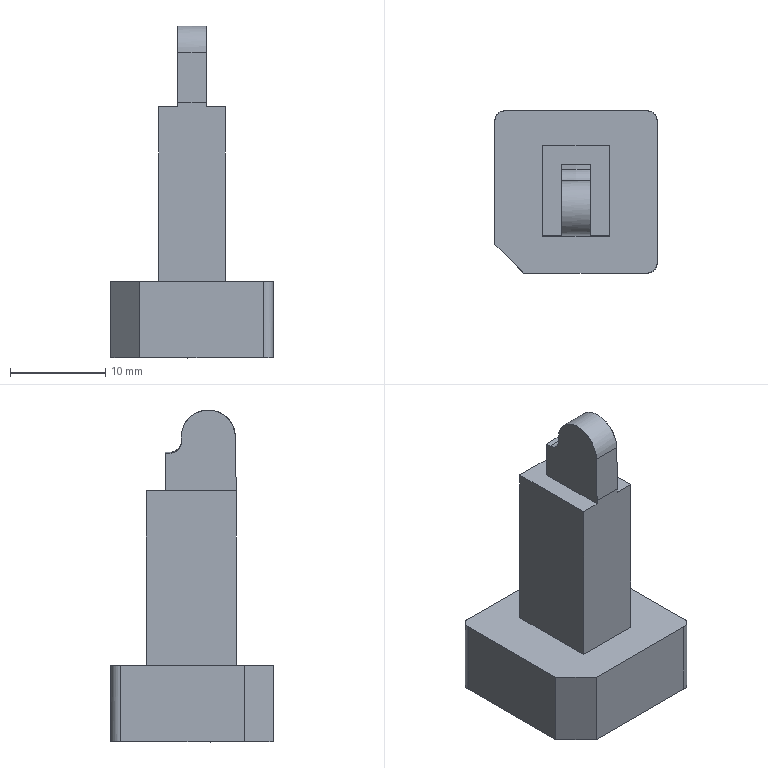NC program | PowerMill | posted with a generic post | part box 17 x 17 x 34.811 mm
Lines 20352 to 21135 of 55221:
N20449 M6
N20450 S18000 M03
N20451 G00 G90 X0.0 Y0.0
N20452 G43 Z10.798 H14
N20453
N20454 G05 P10000 R8
N20455 X2.8132 Y-4.4417
N20456 Z0.9995
N20457 G01 Z-0.2005 F1200.0
N20458 X2.7986 Y-4.3934 F2000.0
N20459 X2.7803 Y-4.3463
N20460 X2.7582 Y-4.3008
N20461 X2.7327 Y-4.2572
N20462 X2.7037 Y-4.2157
N20463 X2.6716 Y-4.1767
N20464 X2.6366 Y-4.1403
N20465 X2.5987 Y-4.1068
N20466 X2.5584 Y-4.0764
N20467 X2.5158 Y-4.0493
N20468 X2.4711 Y-4.0256
N20469 X2.4248 Y-4.0055
N20470 X2.377 Y-3.9892
N20471 X2.3281 Y-3.9766
N20472 X2.2782 Y-3.968
N20473 X2.2279 Y-3.9633
N20474 X2.1774 Y-3.9626
N20475 X2.127 Y-3.9658
N20476 X2.077 Y-3.9731
N20477 X2.0331 Y-3.9828
N20478 X1.9465 Y-4.0053
N20479 X1.8628 Y-4.0231
N20480 X1.783 Y-4.0364
N20481 X1.7026 Y-4.0459
N20482 X1.6159 Y-4.0523
N20483 X1.519 Y-4.0557
N20484 X1.4057 Y-4.0562
N20485 X0.4884 Y-4.0561
N20486 X-0.7174 Y-4.056
N20487 X-1.4208 Y-4.0571
N20488 X-1.5008 Y-4.0569
N20489 X-1.5823 Y-4.0547
N20490 X-1.6674 Y-4.0493
N20491 X-1.7533 Y-4.0404
N20492 X-1.8337 Y-4.0283
N20493 X-1.9109 Y-4.0133
N20494 X-1.9876 Y-3.9951
N20495 X-2.0635 Y-3.9738
N20496 X-2.1466 Y-3.9467
N20497 X-2.2284 Y-3.9158
N20498 X-2.3087 Y-3.8813
N20499 X-2.3874 Y-3.843
N20500 X-2.4643 Y-3.8012
N20501 X-2.5393 Y-3.756
N20502 X-2.6122 Y-3.7073
N20503 X-2.6827 Y-3.6553
N20504 X-2.7508 Y-3.6002
N20505 X-2.8164 Y-3.5421
N20506 X-2.8792 Y-3.481
N20507 X-2.9392 Y-3.4171
N20508 X-2.9963 Y-3.3505
N20509 X-3.0503 Y-3.2815
N20510 X-3.1009 Y-3.2102
N20511 X-3.1484 Y-3.1366
N20512 X-3.1924 Y-3.0609
N20513 X-3.2329 Y-2.9833
N20514 X-3.2699 Y-2.9038
N20515 X-3.3033 Y-2.8227
N20516 X-3.3329 Y-2.7401
N20517 X-3.3587 Y-2.6562
N20518 X-3.3807 Y-2.5713
N20519 X-3.3988 Y-2.4855
N20520 X-3.413 Y-2.3988
N20521 X-3.4232 Y-2.3121
N20522 X-3.4294 Y-2.2257
N20523 X-3.4316 Y-2.1396
N20524 X-3.4317 Y-2.0535
N20525 X-3.4323 Y-1.3276
N20526 X-3.4307 Y-1.2334
N20527 X-3.4253 Y-1.1417
N20528 X-3.4161 Y-1.0522
N20529 X-3.4033 Y-0.9649
N20530 X-3.3868 Y-0.8795
N20531 X-3.3667 Y-0.7958
N20532 X-3.3429 Y-0.7138
N20533 X-3.3156 Y-0.6333
N20534 X-3.2838 Y-0.5518
N20535 X-3.2483 Y-0.4718
N20536 X-3.2092 Y-0.3935
N20537 X-3.1666 Y-0.3171
N20538 X-3.1205 Y-0.2426
N20539 X-3.0711 Y-0.1702
N20540 X-3.0184 Y-0.1002
N20541 X-2.9625 Y-0.0325
N20542 X-2.9036 Y0.0325
N20543 X-2.8418 Y0.0948
N20544 X-2.7773 Y0.1542
N20545 X-2.7101 Y0.2106
N20546 X-2.6405 Y0.2638
N20547 X-2.5686 Y0.3137
N20548 X-2.4946 Y0.3603
N20549 X-2.4185 Y0.4035
N20550 X-2.3405 Y0.4431
N20551 X-2.2608 Y0.4792
N20552 X-2.1795 Y0.5116
N20553 X-2.1011 Y0.5389
N20554 X-2.0215 Y0.5628
N20555 X-1.9398 Y0.5833
N20556 X-1.8556 Y0.6004
N20557 X-1.7687 Y0.614
N20558 X-1.6787 Y0.6242
N20559 X-1.5853 Y0.6308
N20560 X-1.4884 Y0.634
N20561 X-1.3882 Y0.6342
N20562 X0.0 Y0.6333
N20563 X0.8605 Y0.6327
N20564 X1.4431 Y0.6342
N20565 X1.5395 Y0.6331
N20566 X1.6329 Y0.6284
N20567 X1.7234 Y0.6202
N20568 X1.811 Y0.6084
N20569 X1.8959 Y0.5931
N20570 X1.9784 Y0.5743
N20571 X2.0587 Y0.5522
N20572 X2.1376 Y0.5268
N20573 X2.2195 Y0.4963
N20574 X2.2999 Y0.4621
N20575 X2.3788 Y0.4243
N20576 X2.4559 Y0.3828
N20577 X2.5312 Y0.3378
N20578 X2.6044 Y0.2894
N20579 X2.6752 Y0.2378
N20580 X2.7437 Y0.1829
N20581 X2.8097 Y0.125
N20582 X2.873 Y0.0641
N20583 X2.9334 Y0.0004
N20584 X2.9909 Y-0.0659
N20585 X3.0452 Y-0.1347
N20586 X3.0962 Y-0.2058
N20587 X3.1439 Y-0.2791
N20588 X3.1882 Y-0.3544
N20589 X3.229 Y-0.4317
N20590 X3.2662 Y-0.5107
N20591 X3.2988 Y-0.589
N20592 X3.3279 Y-0.6691
N20593 X3.3544 Y-0.7532
N20594 X3.3782 Y-0.842
N20595 X3.3898 Y-0.8923
N20596 X3.3997 Y-0.9429
N20597 X3.4083 Y-0.9938
N20598 X3.4176 Y-1.0584
N20599 X3.4236 Y-1.1096
N20600 X3.428 Y-1.161
N20601 X3.4301 Y-1.2124
N20602 X3.4314 Y-1.4233
N20603 X3.4316 Y-1.6341
N20604 X3.4319 Y-2.069
N20605 X3.4316 Y-2.1567
N20606 X3.4284 Y-2.2443
N20607 X3.4212 Y-2.3316
N20608 X3.4101 Y-2.4185
N20609 X3.395 Y-2.5049
N20610 X3.3761 Y-2.5904
N20611 X3.3532 Y-2.6751
N20612 X3.3265 Y-2.7586
N20613 X3.296 Y-2.8409
N20614 X3.2618 Y-2.9218
N20615 X3.224 Y-3.001
N20616 X3.1826 Y-3.0783
N20617 X3.1377 Y-3.1537
N20618 X3.0895 Y-3.2269
N20619 X3.038 Y-3.2978
N20620 X2.9834 Y-3.3663
N20621 X2.9256 Y-3.4322
N20622 X2.865 Y-3.4955
N20623 X2.8021 Y-3.5554
N20624 X2.7364 Y-3.6125
N20625 X2.6678 Y-3.6668
N20626 X2.5966 Y-3.7181
N20627 X2.523 Y-3.7662
N20628 X2.4473 Y-3.8109
N20629 X2.3697 Y-3.8521
N20630 X2.2906 Y-3.8896
N20631 X2.2101 Y-3.9233
N20632 X2.1286 Y-3.9531
N20633 X2.0463 Y-3.9791
N20634 X2.0331 Y-3.9828
N20635 X1.966 Y-3.9991 Z-0.2006
N20636 X1.8865 Y-4.0194 Z-0.2008
N20637 X1.829 Y-4.0318 Z-0.2009
N20638 X1.7787 Y-4.0395 Z-0.201
N20639 X1.7019 Y-4.0486 Z-0.2011
N20640 X1.6249 Y-4.0557 Z-0.2012
N20641 X1.5477 Y-4.0603 Z-0.2014
N20642 X1.4703 Y-4.0624 Z-0.2015
N20643 X1.3929 Y-4.0631 Z-0.2016
N20644 X1.3156 Y-4.0633 Z-0.2017
N20645 X1.0153 Y-4.0654 Z-0.2022
N20646 X0.6051 Y-4.0709 Z-0.2029
N20647 X0.0021 Y-4.0775 Z-0.2039
N20648 X-0.8982 Y-4.087 Z-0.2055
N20649 X-1.4433 Y-4.0936 Z-0.2065
N20650 X-1.511 Y-4.094 Z-0.2066
N20651 X-1.5788 Y-4.0932 Z-0.2067
N20652 X-1.6466 Y-4.0905 Z-0.2068
N20653 X-1.7141 Y-4.0853 Z-0.2069
N20654 X-1.7814 Y-4.0772 Z-0.207
N20655 X-1.8483 Y-4.0666 Z-0.2071
N20656 X-1.9149 Y-4.0541 Z-0.2072
N20657 X-1.9965 Y-4.0357 Z-0.2073
N20658 X-2.071 Y-4.0153 Z-0.2075
N20659 X-2.1433 Y-3.992 Z-0.2076
N20660 X-2.2174 Y-3.9654 Z-0.2078
N20661 X-2.2904 Y-3.9357 Z-0.2079
N20662 X-2.362 Y-3.9028 Z-0.208
N20663 X-2.4321 Y-3.8669 Z-0.2081
N20664 X-2.5007 Y-3.8282 Z-0.2083
N20665 X-2.5678 Y-3.787 Z-0.2084
N20666 X-2.6395 Y-3.7385 Z-0.2086
N20667 X-2.7087 Y-3.6868 Z-0.2088
N20668 X-2.7756 Y-3.632 Z-0.209
N20669 X-2.84 Y-3.574 Z-0.2092
N20670 X-2.9019 Y-3.5128 Z-0.2094
N20671 X-2.9612 Y-3.4486 Z-0.2095
N20672 X-3.018 Y-3.3817 Z-0.2098
N20673 X-3.0726 Y-3.3118 Z-0.2102
N20674 X-3.1218 Y-3.2428 Z-0.2107
N20675 X-3.1658 Y-3.1745 Z-0.2112
N20676 X-3.2051 Y-3.1066 Z-0.2116
N20677 X-3.2406 Y-3.0378 Z-0.2118
N20678 X-3.2766 Y-2.9596 Z-0.2119
N20679 X-3.3094 Y-2.8787 Z-0.2121
N20680 X-3.3389 Y-2.7954 Z-0.2122
N20681 X-3.3606 Y-2.7254 Z-0.2124
N20682 X-3.3768 Y-2.6644 Z-0.2125
N20683 X-3.3906 Y-2.6028 Z-0.2127
N20684 X-3.4025 Y-2.5408 Z-0.2128
N20685 X-3.4148 Y-2.4634 Z-0.2129
N20686 X-3.4241 Y-2.3861 Z-0.2131
N20687 X-3.4291 Y-2.3233 Z-0.2132
N20688 X-3.4313 Y-2.2603 Z-0.2133
N20689 X-3.4314 Y-2.1972 Z-0.2134
N20690 X-3.4319 Y-1.2121 Z-0.2154
N20691 X-3.43 Y-1.122 Z-0.2155
N20692 X-3.4241 Y-1.0323 Z-0.2157
N20693 X-3.4142 Y-0.9433 Z-0.2159
N20694 X-3.4005 Y-0.8551 Z-0.2161
N20695 X-3.3829 Y-0.7679 Z-0.2163
N20696 X-3.3614 Y-0.6819 Z-0.2165
N20697 X-3.3362 Y-0.5974 Z-0.2167
N20698 X-3.3074 Y-0.5144 Z-0.2169
N20699 X-3.2749 Y-0.4331 Z-0.217
N20700 X-3.2389 Y-0.3538 Z-0.2171
N20701 X-3.1995 Y-0.2764
N20702 X-3.166 Y-0.2173
N20703 X-3.1298 Y-0.1598 Z-0.217
N20704 X-3.0917 Y-0.1036 Z-0.2169
N20705 X-3.0468 Y-0.0419 Z-0.2168
N20706 X-2.9903 Y0.0304 Z-0.2167
N20707 X-2.9408 Y0.0888
N20708 X-2.8949 Y0.1389 Z-0.2168
N20709 X-2.8472 Y0.1872 Z-0.217
N20710 X-2.7836 Y0.2463 Z-0.2171
N20711 X-2.7146 Y0.3051 Z-0.2172
N20712 X-2.649 Y0.3569 Z-0.2173
N20713 X-2.5812 Y0.4058 Z-0.2174
N20714 X-2.5103 Y0.4521 Z-0.2175
N20715 X-2.4362 Y0.4957 Z-0.2177
N20716 X-2.3591 Y0.5366 Z-0.2179
N20717 X-2.2788 Y0.5746 Z-0.218
N20718 X-2.1956 Y0.6096 Z-0.2182
N20719 X-2.1095 Y0.6416 Z-0.2184
N20720 X-2.0323 Y0.6663 Z-0.2185
N20721 X-1.9511 Y0.6882 Z-0.2187
N20722 X-1.872 Y0.706 Z-0.2188
N20723 X-1.7922 Y0.7206 Z-0.219
N20724 X-1.7119 Y0.7319 Z-0.2192
N20725 X-1.6306 Y0.7398 Z-0.2193
N20726 X-1.5402 Y0.7449 Z-0.2195
N20727 X-1.459 Y0.7469 Z-0.2197
N20728 X-1.3773 Y0.7475 Z-0.2199
N20729 X-0.5456 Y0.7553 Z-0.2215
N20730 X0.6708 Y0.7679 Z-0.2239
N20731 X1.3606 Y0.7761 Z-0.2255
N20732 X1.4438 Y0.7773 Z-0.2257
N20733 X1.5235 Y0.7775 Z-0.2258
N20734 X1.6031 Y0.7752 Z-0.226
N20735 X1.6834 Y0.7701 Z-0.2262
N20736 X1.7655 Y0.7616 Z-0.2263
N20737 X1.8494 Y0.7492 Z-0.2265
N20738 X1.9326 Y0.733 Z-0.2267
N20739 X2.0128 Y0.7137 Z-0.2269
N20740 X2.0903 Y0.6916 Z-0.2271
N20741 X2.1737 Y0.6642 Z-0.2273
N20742 X2.2543 Y0.6336 Z-0.2275
N20743 X2.3321 Y0.5998 Z-0.2277
N20744 X2.4072 Y0.563 Z-0.2279
N20745 X2.4798 Y0.5231 Z-0.2281
N20746 X2.5563 Y0.4764 Z-0.2283
N20747 X2.6301 Y0.4269 Z-0.2285
N20748 X2.701 Y0.3745 Z-0.2287
N20749 X2.7691 Y0.3194 Z-0.229
N20750 X2.8343 Y0.2614 Z-0.2292
N20751 X2.8965 Y0.2007 Z-0.2295
N20752 X2.9559 Y0.1372 Z-0.2298
N20753 X3.0124 Y0.0711 Z-0.2301
N20754 X3.0659 Y0.0023 Z-0.2305
N20755 X3.1164 Y-0.0692 Z-0.2309
N20756 X3.1612 Y-0.1389 Z-0.2313
N20757 X3.2027 Y-0.2111 Z-0.2315
N20758 X3.241 Y-0.2856 Z-0.2316
N20759 X3.2759 Y-0.3623 Z-0.2318
N20760 X3.3075 Y-0.4411 Z-0.2319
N20761 X3.338 Y-0.5268 Z-0.2321
N20762 X3.3628 Y-0.6066 Z-0.2322
N20763 X3.3824 Y-0.6819 Z-0.2324
N20764 X3.3974 Y-0.7536 Z-0.2325
N20765 X3.4078 Y-0.817 Z-0.2327
N20766 X3.4167 Y-0.8806 Z-0.2328
N20767 X3.4238 Y-0.9443 Z-0.2329
N20768 X3.4288 Y-1.0083 Z-0.2331
N20769 X3.4315 Y-1.0732 Z-0.2332
N20770 X3.4325 Y-1.1376 Z-0.2333
N20771 X3.4324 Y-1.2019 Z-0.2334
N20772 X3.4319 Y-1.2663 Z-0.2336
N20773 X3.4317 Y-1.3306 Z-0.2337
N20774 X3.4315 Y-1.7185 Z-0.2345
N20775 X3.4328 Y-2.0772 Z-0.2352
N20776 X3.432 Y-2.3058 Z-0.2356
N20777 X3.4308 Y-2.3895 Z-0.2358
N20778 X3.4264 Y-2.4733 Z-0.2359
N20779 X3.4181 Y-2.5577 Z-0.2361
N20780 X3.4057 Y-2.6427 Z-0.2363
N20781 X3.3893 Y-2.7282 Z-0.2365
N20782 X3.3687 Y-2.8139 Z-0.2366
N20783 X3.3441 Y-2.8997 Z-0.2368
N20784 X3.3153 Y-2.9855 Z-0.237
N20785 X3.2841 Y-3.0669 Z-0.2371
N20786 X3.2493 Y-3.1468 Z-0.2373
N20787 X3.2108 Y-3.2253 Z-0.2375
N20788 X3.1687 Y-3.302 Z-0.2377
N20789 X3.1231 Y-3.3769 Z-0.2379
N20790 X3.074 Y-3.4498 Z-0.238
N20791 X3.0221 Y-3.5199 Z-0.2382
N20792 X2.967 Y-3.5875 Z-0.2383
N20793 X2.9085 Y-3.653 Z-0.2384
N20794 X2.8467 Y-3.7163 Z-0.2386
N20795 X2.7817 Y-3.7772 Z-0.2387
N20796 X2.7135 Y-3.8355 Z-0.2389
N20797 X2.6546 Y-3.8819 Z-0.239
N20798 X2.5921 Y-3.9269 Z-0.2392
N20799 X2.5227 Y-3.9726 Z-0.2394
N20800 X2.4473 Y-4.0178 Z-0.2396
N20801 X2.3687 Y-4.0604 Z-0.2398
N20802 X2.2915 Y-4.0979 Z-0.2399
N20803 X2.2177 Y-4.1299 Z-0.2401
N20804 X2.1477 Y-4.1566 Z-0.2403
N20805 X2.0929 Y-4.1749 Z-0.2405
N20806 X2.0149 Y-4.1995 Z-0.2406
N20807 X1.9428 Y-4.2186 Z-0.2407
N20808 X1.8756 Y-4.2331 Z-0.2409
N20809 X1.8081 Y-4.2455 Z-0.241
N20810 X1.7403 Y-4.2558 Z-0.2411
N20811 X1.6721 Y-4.2636 Z-0.2412
N20812 X1.6036 Y-4.2686 Z-0.2414
N20813 X1.5349 Y-4.2712 Z-0.2415
N20814 X1.4661 Y-4.2722 Z-0.2416
N20815 X1.3973 Y-4.2723 Z-0.2417
N20816 X1.3286 Y-4.2722 Z-0.2418
N20817 X1.0522 Y-4.2739 Z-0.2422
N20818 X0.7391 Y-4.2771 Z-0.2428
N20819 X-0.0765 Y-4.2834 Z-0.2443
N20820 X-0.609 Y-4.2876 Z-0.2453
N20821 X-1.0303 Y-4.2904 Z-0.2461
N20822 X-1.4432 Y-4.2949 Z-0.2468
N20823 X-1.5335 Y-4.2948 Z-0.247
N20824 X-1.6229 Y-4.2915 Z-0.2472
N20825 X-1.7112 Y-4.2847 Z-0.2473
N20826 X-1.7982 Y-4.2743 Z-0.2475
N20827 X-1.8833 Y-4.2601 Z-0.2476
N20828 X-1.9665 Y-4.2424 Z-0.2477
N20829 X-2.0479 Y-4.2211 Z-0.2479
N20830 X-2.1276 Y-4.1963 Z-0.248
N20831 X-2.2068 Y-4.1679 Z-0.2482
N20832 X-2.2884 Y-4.1346 Z-0.2484
N20833 X-2.3675 Y-4.0981 Z-0.2485
N20834 X-2.4445 Y-4.0582 Z-0.2487
N20835 X-2.5199 Y-4.0147 Z-0.2489
N20836 X-2.5931 Y-3.9677 Z-0.2491
N20837 X-2.6641 Y-3.9174 Z-0.2492
N20838 X-2.7321 Y-3.8645 Z-0.2494
N20839 X-2.8019 Y-3.8053 Z-0.2497
N20840 X-2.8643 Y-3.7476 Z-0.2501
N20841 X-2.9204 Y-3.6908 Z-0.2504
N20842 X-2.972 Y-3.6333 Z-0.2506
N20843 X-3.0272 Y-3.5658 Z-0.2507
N20844 X-3.0794 Y-3.4957 Z-0.2508
N20845 X-3.1286 Y-3.4231 Z-0.251
N20846 X-3.1745 Y-3.3481 Z-0.2512
N20847 X-3.217 Y-3.271 Z-0.2513
N20848 X-3.2562 Y-3.1918 Z-0.2515
N20849 X-3.2891 Y-3.1169 Z-0.2517
N20850 X-3.319 Y-3.0392 Z-0.2518
N20851 X-3.3465 Y-2.9572 Z-0.252
N20852 X-3.3714 Y-2.8703 Z-0.2522
N20853 X-3.3825 Y-2.8265
N20854 X-3.392 Y-2.7823 Z-0.2523
N20855 X-3.4004 Y-2.7378 Z-0.2524
N20856 X-3.408 Y-2.6922 Z-0.2525
N20857 X-3.4175 Y-2.6273 Z-0.2526
N20858 X-3.4239 Y-2.5733 Z-0.2527
N20859 X-3.4279 Y-2.5283 Z-0.2528
N20860 X-3.4298 Y-2.4832 Z-0.2529
N20861 X-3.4301 Y-2.438 Z-0.253
N20862 X-3.4312 Y-1.8823 Z-0.2541
N20863 X-3.4318 Y-1.2727 Z-0.2552
N20864 X-3.4311 Y-0.9812 Z-0.2558
N20865 X-3.4288 Y-0.9046 Z-0.2559
N20866 X-3.4229 Y-0.8282 Z-0.2561
N20867 X-3.4132 Y-0.7479 Z-0.2562
N20868 X-3.3993 Y-0.6639 Z-0.2564
N20869 X-3.3811 Y-0.5772 Z-0.2565
N20870 X-3.3588 Y-0.4898 Z-0.2567
N20871 X-3.3331 Y-0.4051 Z-0.2569
N20872 X-3.3047 Y-0.3246 Z-0.257
N20873 X-3.2742 Y-0.249 Z-0.2572
N20874 X-3.2413 Y-0.177 Z-0.2573
N20875 X-3.2005 Y-0.0966 Z-0.2575
N20876 X-3.1568 Y-0.019 Z-0.2577
N20877 X-3.1102 Y0.0556 Z-0.2579
N20878 X-3.0608 Y0.1271 Z-0.2581
N20879 X-3.0089 Y0.1955 Z-0.2582
N20880 X-2.9543 Y0.2609 Z-0.2583
N20881 X-2.8952 Y0.3255 Z-0.2584
N20882 X-2.8334 Y0.3873
N20883 X-2.769 Y0.4461 Z-0.2585
N20884 X-2.7018 Y0.5021
N20885 X-2.6318 Y0.5552 Z-0.2586
N20886 X-2.5589 Y0.6056 Z-0.2587
N20887 X-2.4831 Y0.6531 Z-0.2589
N20888 X-2.4042 Y0.6979 Z-0.259
N20889 X-2.3349 Y0.7333 Z-0.2592
N20890 X-2.2589 Y0.7678 Z-0.2593
N20891 X-2.1829 Y0.7987 Z-0.2594
N20892 X-2.1055 Y0.8268 Z-0.2596
N20893 X-2.0263 Y0.8516 Z-0.2598
N20894 X-1.9451 Y0.873 Z-0.2599
N20895 X-1.8615 Y0.8909 Z-0.2601
N20896 X-1.7754 Y0.9054 Z-0.2602
N20897 X-1.6864 Y0.9164 Z-0.2604
N20898 X-1.5942 Y0.9238 Z-0.2606
N20899 X-1.4985 Y0.9277 Z-0.2608
N20900 X-1.3995 Y0.9285 Z-0.261
N20901 X-0.8488 Y0.9315 Z-0.2621
N20902 X-0.0933 Y0.9375 Z-0.2635
N20903 X0.652 Y0.9427 Z-0.2649
N20904 X1.4437 Y0.9495 Z-0.2664
N20905 X1.5217 Y0.9494 Z-0.2665
N20906 X1.5998 Y0.9472 Z-0.2666
N20907 X1.6777 Y0.9424 Z-0.2668
N20908 X1.7575 Y0.9344 Z-0.267
N20909 X1.8406 Y0.9223 Z-0.2672
N20910 X1.9172 Y0.9077 Z-0.2673
N20911 X1.9933 Y0.8902 Z-0.2675
N20912 X2.0686 Y0.8698 Z-0.2677
N20913 X2.1474 Y0.8445 Z-0.2678
N20914 X2.2275 Y0.8146 Z-0.2679
N20915 X2.3091 Y0.78 Z-0.2681
N20916 X2.3824 Y0.7453 Z-0.2683
N20917 X2.4555 Y0.7067 Z-0.2684
N20918 X2.5296 Y0.6632 Z-0.2687
N20919 X2.6037 Y0.6152 Z-0.2689
N20920 X2.676 Y0.5636 Z-0.2692
N20921 X2.7446 Y0.5099 Z-0.2695
N20922 X2.8086 Y0.455 Z-0.2698
N20923 X2.8681 Y0.3991 Z-0.27
N20924 X2.9248 Y0.3404 Z-0.2702
N20925 X2.9819 Y0.2758 Z-0.2704
N20926 X3.0384 Y0.206 Z-0.2706
N20927 X3.0862 Y0.1414 Z-0.2707
N20928 X3.1318 Y0.0729 Z-0.2709
N20929 X3.1758 Y0.0 Z-0.2711
N20930 X3.218 Y-0.0777 Z-0.2712
N20931 X3.2588 Y-0.1609 Z-0.2714
N20932 X3.2881 Y-0.2265 Z-0.2715
N20933 X3.3149 Y-0.2949 Z-0.2717
N20934 X3.3407 Y-0.3712 Z-0.2718
N20935 X3.3665 Y-0.459 Z-0.272
N20936 X3.3833 Y-0.5223 Z-0.2721
N20937 X3.3912 Y-0.558 Z-0.2722
N20938 X3.398 Y-0.594 Z-0.2723
N20939 X3.4041 Y-0.63
N20940 X3.4113 Y-0.6772 Z-0.2724
N20941 X3.4201 Y-0.7436 Z-0.2725
N20942 X3.425 Y-0.7884 Z-0.2726
N20943 X3.428 Y-0.8247 Z-0.2727
N20944 X3.4298 Y-0.8612 Z-0.2728
N20945 X3.4301 Y-0.8978
N20946 X3.4315 Y-1.2847 Z-0.2736
N20947 X3.4318 Y-1.9852 Z-0.2749
N20948 X3.4317 Y-2.4843 Z-0.2759
N20949 X3.4296 Y-2.5722 Z-0.276
N20950 X3.4235 Y-2.66 Z-0.2762
N20951 X3.4135 Y-2.7475 Z-0.2764
N20952 X3.3994 Y-2.8345 Z-0.2765
N20953 X3.3814 Y-2.9209 Z-0.2767
N20954 X3.3595 Y-3.0065 Z-0.2769
N20955 X3.3338 Y-3.091 Z-0.277
N20956 X3.3042 Y-3.1744 Z-0.2772
N20957 X3.2709 Y-3.2563 Z-0.2774
N20958 X3.2341 Y-3.3363 Z-0.2775
N20959 X3.1937 Y-3.4145 Z-0.2777
N20960 X3.1499 Y-3.4908 Z-0.2779
N20961 X3.1025 Y-3.5651 Z-0.2781
N20962 X3.0518 Y-3.6373 Z-0.2782
N20963 X2.9979 Y-3.7071 Z-0.2784
N20964 X2.9408 Y-3.7745 Z-0.2786
N20965 X2.8807 Y-3.8392 Z-0.2787
N20966 X2.8193 Y-3.8996 Z-0.2789
N20967 X2.755 Y-3.9575 Z-0.279
N20968 X2.6873 Y-4.0131 Z-0.2792
N20969 X2.6166 Y-4.0659 Z-0.2794
N20970 X2.5433 Y-4.1158 Z-0.2795
N20971 X2.468 Y-4.1622 Z-0.2797
N20972 X2.3911 Y-4.2049 Z-0.2799
N20973 X2.3131 Y-4.2437 Z-0.28
N20974 X2.2345 Y-4.2784 Z-0.2802
N20975 X2.1556 Y-4.309 Z-0.2804
N20976 X2.1455 Y-4.3126
N20977 X2.0746 Y-4.3369 Z-0.2805
N20978 X1.997 Y-4.3594 Z-0.2807
N20979 X1.9108 Y-4.3805 Z-0.2808
N20980 X1.8314 Y-4.3964 Z-0.281
N20981 X1.7482 Y-4.4091 Z-0.2811
N20982 X1.6603 Y-4.4186 Z-0.2813
N20983 X1.5668 Y-4.4248 Z-0.2814
N20984 X1.4667 Y-4.4275 Z-0.2816
N20985 X1.358 Y-4.4278 Z-0.2818
N20986 X0.6883 Y-4.431 Z-0.283
N20987 X0.0184 Y-4.436 Z-0.2842
N20988 X-0.6822 Y-4.4399 Z-0.2854
N20989 X-1.3754 Y-4.4439 Z-0.2866
N20990 X-1.4809 Y-4.4446 Z-0.2868
N20991 X-1.5811 Y-4.4427 Z-0.287
N20992 X-1.6739 Y-4.4374 Z-0.2871
N20993 X-1.7602 Y-4.429 Z-0.2873
N20994 X-1.8445 Y-4.4169 Z-0.2874
N20995 X-1.9249 Y-4.4016 Z-0.2876
N20996 X-2.0048 Y-4.3826 Z-0.2878
N20997 X-2.0865 Y-4.3591 Z-0.288
N20998 X-2.1693 Y-4.3313 Z-0.2882
N20999 X-2.2522 Y-4.2992 Z-0.2884
N21000 X-2.3335 Y-4.2635 Z-0.2886
N21001 X-2.4118 Y-4.2249 Z-0.2888
N21002 X-2.4862 Y-4.184 Z-0.289
N21003 X-2.556 Y-4.1413 Z-0.2892
N21004 X-2.6238 Y-4.0955 Z-0.2894
N21005 X-2.6931 Y-4.0444 Z-0.2896
N21006 X-2.758 Y-3.9918 Z-0.2897
N21007 X-2.8233 Y-3.9338 Z-0.2899
N21008 X-2.886 Y-3.8728 Z-0.29
N21009 X-2.9458 Y-3.809 Z-0.2902
N21010 X-3.0025 Y-3.7427 Z-0.2904
N21011 X-3.0562 Y-3.6738 Z-0.2905
N21012 X-3.1065 Y-3.6027 Z-0.2907
N21013 X-3.1527 Y-3.5307 Z-0.2909
N21014 X-3.1956 Y-3.4566 Z-0.291
N21015 X-3.2358 Y-3.3794 Z-0.2912
N21016 X-3.2732 Y-3.2988 Z-0.2913
N21017 X-3.3078 Y-3.2149 Z-0.2915
N21018 X-3.3299 Y-3.1551 Z-0.2916
N21019 X-3.3494 Y-3.0943 Z-0.2917
N21020 X-3.3667 Y-3.0329 Z-0.2919
N21021 X-3.3829 Y-2.9671 Z-0.292
N21022 X-3.3993 Y-2.889 Z-0.2921
N21023 X-3.4138 Y-2.8038 Z-0.2923
N21024 X-3.4232 Y-2.7294 Z-0.2924
N21025 X-3.4286 Y-2.6648 Z-0.2926
N21026 X-3.4308 Y-2.6012 Z-0.2927
N21027 X-3.431 Y-2.5374 Z-0.2928
N21028 X-3.4316 Y-1.7894 Z-0.2942
N21029 Y-0.9962 Z-0.2957
N21030 X-3.4314 Y-0.8658 Z-0.2959
N21031 X-3.4292 Y-0.778 Z-0.2961
N21032 X-3.423 Y-0.6905 Z-0.2962
N21033 X-3.4128 Y-0.6033 Z-0.2964
N21034 X-3.3987 Y-0.5166 Z-0.2966
N21035 X-3.3806 Y-0.4305 Z-0.2967
N21036 X-3.3586 Y-0.3452 Z-0.2969
N21037 X-3.3328 Y-0.261 Z-0.297
N21038 X-3.3031 Y-0.178 Z-0.2972
N21039 X-3.2697 Y-0.0964 Z-0.2974
N21040 X-3.2327 Y-0.0164 Z-0.2975
N21041 X-3.1921 Y0.0618 Z-0.2977
N21042 X-3.1479 Y0.1382 Z-0.2978
N21043 X-3.1004 Y0.2125 Z-0.298
N21044 X-3.0495 Y0.2846 Z-0.2982
N21045 X-2.9954 Y0.3543 Z-0.2983
N21046 X-2.9383 Y0.4214 Z-0.2985
N21047 X-2.8782 Y0.4858 Z-0.2987
N21048 X-2.8154 Y0.5473 Z-0.2989
N21049 X-2.7499 Y0.6059 Z-0.299
N21050 X-2.6819 Y0.6614 Z-0.2992
N21051 X-2.6115 Y0.7136 Z-0.2993
N21052 X-2.5388 Y0.7626 Z-0.2995
N21053 X-2.464 Y0.8082 Z-0.2996
N21054 X-2.3873 Y0.8503 Z-0.2997
N21055 X-2.3088 Y0.8888 Z-0.2998
N21056 X-2.2287 Y0.9237 Z-0.2999
N21057 X-2.1473 Y0.9548 Z-0.3
N21058 X-2.0646 Y0.9821 Z-0.3001
N21059 X-1.9925 Y1.0025 Z-0.3002
N21060 X-1.9197 Y1.0205 Z-0.3003
N21061 X-1.8463 Y1.0357 Z-0.3004
N21062 X-1.7723 Y1.0479 Z-0.3005
N21063 X-1.6907 Y1.0577 Z-0.3007
N21064 X-1.6142 Y1.0637 Z-0.3008
N21065 X-1.5392 Y1.067 Z-0.3009
N21066 X-1.4642 Y1.0685 Z-0.3011
N21067 X-1.3891 Y1.0689 Z-0.3013
N21068 X0.4892 Y1.0791 Z-0.3049
N21069 X1.4436 Y1.0854 Z-0.3066
N21070 X1.5213 Y1.0851 Z-0.3068
N21071 X1.5992 Y1.0828 Z-0.3069
N21072 X1.6814 Y1.0776 Z-0.3071
N21073 X1.7666 Y1.0686 Z-0.3073
N21074 X1.846 Y1.0567 Z-0.3075
N21075 X1.9222 Y1.0418 Z-0.3077
N21076 X1.9978 Y1.0238 Z-0.3078
N21077 X2.0727 Y1.0031 Z-0.308
N21078 X2.1549 Y0.9766 Z-0.3082
N21079 X2.2348 Y0.9468 Z-0.3085
N21080 X2.3127 Y0.9135 Z-0.3086
N21081 X2.3916 Y0.8754 Z-0.3088
N21082 X2.468 Y0.8343 Z-0.309
N21083 X2.5416 Y0.7902 Z-0.3091
N21084 X2.6123 Y0.7432 Z-0.3093
N21085 X2.6806 Y0.6931 Z-0.3094
N21086 X2.7495 Y0.6378 Z-0.3096
N21087 X2.8157 Y0.5794 Z-0.3098
N21088 X2.8791 Y0.5183 Z-0.3099
N21089 X2.9395 Y0.4544 Z-0.3101
N21090 X2.9969 Y0.388 Z-0.3103
N21091 X3.0511 Y0.3192 Z-0.3104
N21092 X3.1021 Y0.248 Z-0.3106
N21093 X3.1497 Y0.1746 Z-0.3107
N21094 X3.1936 Y0.0997 Z-0.3109
N21095 X3.2338 Y0.0234 Z-0.3111
N21096 X3.2701 Y-0.0541 Z-0.3112
N21097 X3.3025 Y-0.1327 Z-0.3114
N21098 X3.3311 Y-0.2123 Z-0.3115
N21099 X3.3571 Y-0.2962 Z-0.3117
N21100 X3.3798 Y-0.383 Z-0.3119
N21101 X3.3992 Y-0.4728 Z-0.312
N21102 X3.4136 Y-0.5551 Z-0.3122
N21103 X3.4234 Y-0.6303 Z-0.3123
N21104 X3.4288 Y-0.6978 Z-0.3125
N21105 X3.4304 Y-0.7601 Z-0.3126
N21106 X3.4317 Y-1.0866 Z-0.3132
N21107 X3.4318 Y-1.3942 Z-0.3137
N21108 X3.432 Y-2.5976 Z-0.316
N21109 X3.4301 Y-2.6878 Z-0.3162
N21110 X3.4242 Y-2.7775 Z-0.3163
N21111 X3.4144 Y-2.8666 Z-0.3165
N21112 X3.4006 Y-2.9548 Z-0.3166
N21113 X3.383 Y-3.0419 Z-0.3168
N21114 X3.3616 Y-3.1278 Z-0.317
N21115 X3.3364 Y-3.2124 Z-0.3171
N21116 X3.3075 Y-3.2954 Z-0.3173
N21117 X3.2751 Y-3.3768 Z-0.3175
N21118 X3.239 Y-3.4563 Z-0.3176
N21119 X3.1994 Y-3.5341 Z-0.3178
N21120 X3.156 Y-3.6105 Z-0.318
N21121 X3.1092 Y-3.6849 Z-0.3181
N21122 X3.0589 Y-3.7572 Z-0.3183
N21123 X3.0053 Y-3.8273 Z-0.3184
N21124 X2.9485 Y-3.8951 Z-0.3186
N21125 X2.8886 Y-3.9604 Z-0.3188
N21126 X2.8256 Y-4.023 Z-0.3189
N21127 X2.7667 Y-4.0766 Z-0.3191
N21128 X2.7023 Y-4.1301 Z-0.3192
N21129 X2.633 Y-4.1828 Z-0.3194
N21130 X2.5598 Y-4.2335 Z-0.3196
N21131 X2.4847 Y-4.2807 Z-0.3197
N21132 X2.4097 Y-4.3233 Z-0.3199
N21133 X2.3357 Y-4.3611 Z-0.32
N21134 X2.2636 Y-4.3938 Z-0.3202
N21135 X2.192 Y-4.4223 Z-0.3203
N21136 X2.1879 Y-4.4238
N21137 X2.112 Y-4.452 Z-0.3205
N21138 X2.0333 Y-4.4771 Z-0.3206
N21139 X1.952 Y-4.4988 Z-0.3208
N21140 X1.8707 Y-4.5166 Z-0.3209
N21141 X1.7875 Y-4.5308 Z-0.3211
N21142 X1.7001 Y-4.5418 Z-0.3213
N21143 X1.608 Y-4.5494 Z-0.3214
N21144 X1.5104 Y-4.5536 Z-0.3216
N21145 X1.4064 Y-4.5544 Z-0.3218
N21146 X0.7617 Y-4.5564 Z-0.323
N21147 X-0.0001 Y-4.5606 Z-0.3243
N21148 X-0.9118 Y-4.565 Z-0.326
N21149 X-1.4432 Y-4.569 Z-0.327
N21150 X-1.5323 Y-4.5685 Z-0.3271
N21151 X-1.6229 Y-4.565 Z-0.3273
N21152 X-1.7123 Y-4.558 Z-0.3274
N21153 X-1.7976 Y-4.5475 Z-0.3276
N21154 X-1.8788 Y-4.5338 Z-0.3278
N21155 X-1.9587 Y-4.5167 Z-0.3279
N21156 X-2.0379 Y-4.4962 Z-0.3281
N21157 X-2.1216 Y-4.4706 Z-0.3282
N21158 X-2.204 Y-4.4411 Z-0.3284
N21159 X-2.2849 Y-4.408 Z-0.3285
N21160 X-2.3643 Y-4.3711 Z-0.3287
N21161 X-2.4419 Y-4.3307 Z-0.3289
N21162 X-2.5176 Y-4.2868 Z-0.329
N21163 X-2.5912 Y-4.2395 Z-0.3292
N21164 X-2.6626 Y-4.1888 Z-0.3293
N21165 X-2.7314 Y-4.1351 Z-0.3295
N21166 X-2.7978 Y-4.0782 Z-0.3296
N21167 X-2.8615 Y-4.0184 Z-0.3298
N21168 X-2.9223 Y-3.9557 Z-0.33
N21169 X-2.9803 Y-3.8903 Z-0.3301
N21170 X-3.0352 Y-3.8224 Z-0.3303
N21171 X-3.0869 Y-3.752 Z-0.3304
N21172 X-3.1354 Y-3.6793 Z-0.3306
N21173 X-3.1804 Y-3.6045 Z-0.3308
N21174 X-3.222 Y-3.5277 Z-0.3309
N21175 X-3.26 Y-3.4491 Z-0.3311
N21176 X-3.2944 Y-3.3689 Z-0.3312
N21177 X-3.3251 Y-3.2872 Z-0.3314
N21178 X-3.3524 Y-3.2037 Z-0.3316
N21179 X-3.3756 Y-3.1204 Z-0.3317
N21180 X-3.3945 Y-3.0376 Z-0.3319
N21181 X-3.4093 Y-2.9554 Z-0.332
N21182 X-3.42 Y-2.8738 Z-0.3322
N21183 X-3.4267 Y-2.793 Z-0.3323
N21184 X-3.4294 Y-2.713 Z-0.3325
N21185 X-3.43 Y-2.6328 Z-0.3326
N21186 X-3.4317 Y-2.1799 Z-0.3334
N21187 X-3.4318 Y-1.4424 Z-0.3348
N21188 X-3.4316 Y-0.7504 Z-0.336
N21189 X-3.4295 Y-0.6625 Z-0.3362
N21190 X-3.4234 Y-0.5747 Z-0.3363
N21191 X-3.4134 Y-0.4874 Z-0.3365
N21192 X-3.3994 Y-0.4006 Z-0.3367
N21193 X-3.3814 Y-0.3144 Z-0.3368
N21194 X-3.3596 Y-0.2292 Z-0.337
N21195 X-3.3339 Y-0.1449 Z-0.3371
N21196 X-3.3043 Y-0.0619 Z-0.3373
N21197 X-3.2711 Y0.0196 Z-0.3375
N21198 X-3.2342 Y0.0996 Z-0.3376
N21199 X-3.1937 Y0.1778 Z-0.3378
N21200 X-3.1498 Y0.2541 Z-0.3379
N21201 X-3.1026 Y0.3281 Z-0.3381
N21202 X-3.052 Y0.3998 Z-0.3383
N21203 X-2.9982 Y0.4693 Z-0.3384
N21204 X-2.9412 Y0.5364 Z-0.3386
N21205 X-2.8811 Y0.6009 Z-0.3387
N21206 X-2.818 Y0.6628 Z-0.3389
N21207 X-2.7522 Y0.7218 Z-0.3391
N21208 X-2.6843 Y0.7772 Z-0.3392
N21209 X-2.614 Y0.8295 Z-0.3394
N21210 X-2.5414 Y0.8786 Z-0.3395
N21211 X-2.4665 Y0.9244 Z-0.3397
N21212 X-2.3896 Y0.9667 Z-0.3399
N21213 X-2.3108 Y1.0055 Z-0.34
N21214 X-2.2302 Y1.0408 Z-0.3402
N21215 X-2.1481 Y1.0723 Z-0.3403
N21216 X-2.0647 Y1.1001 Z-0.3405
N21217 X-1.9802 Y1.124 Z-0.3406
N21218 X-1.8947 Y1.1441 Z-0.3408
N21219 X-1.8085 Y1.1602 Z-0.341
N21220 X-1.7314 Y1.1711 Z-0.3411
N21221 X-1.6491 Y1.1789 Z-0.3412
N21222 X-1.5565 Y1.1839 Z-0.3414
N21223 X-1.4467 Y1.1862 Z-0.3416
N21224 X-1.2954 Y1.1868 Z-0.3419
N21225 X-0.0431 Y1.1926 Z-0.3442
N21226 X0.6565 Y1.1957 Z-0.3454
N21227 X1.1832 Y1.1983 Z-0.3464
N21228 X1.4435 Y1.2006 Z-0.3469
N21229 X1.5377 Y1.2 Z-0.347
N21230 X1.63 Y1.196 Z-0.3472
N21231 X1.7199 Y1.1886 Z-0.3474
N21232 X1.8073 Y1.1775 Z-0.3475